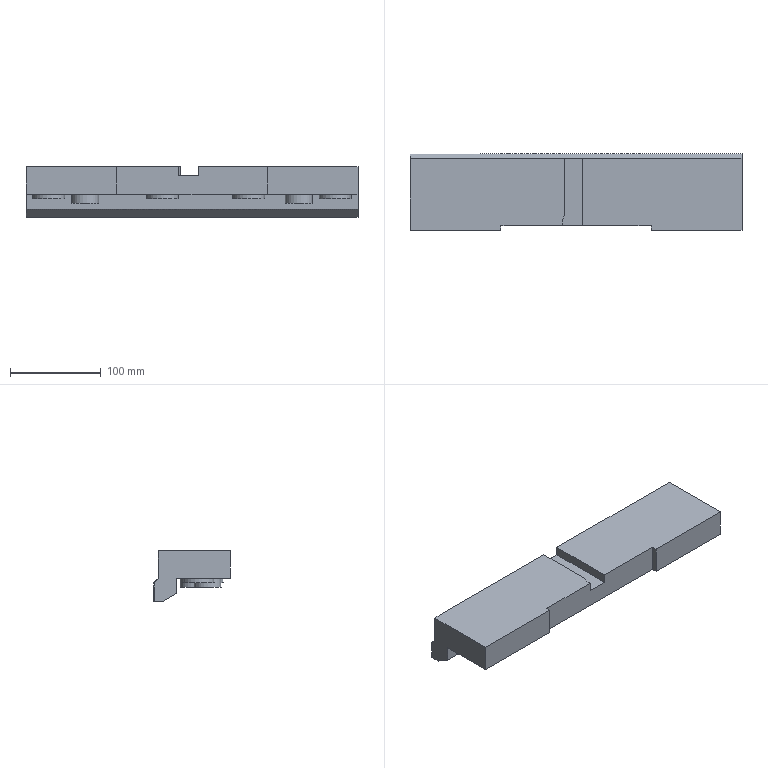Part | NX | features solid 2 | 1 solid | 32 faces | box 365 x 84.391 x 55.35 mm | volume 1065355 mm3 | plane 19 | cylinder 7 | spline 6 | commonest cylinder face diameters 35 x4 30 x2 25 x1